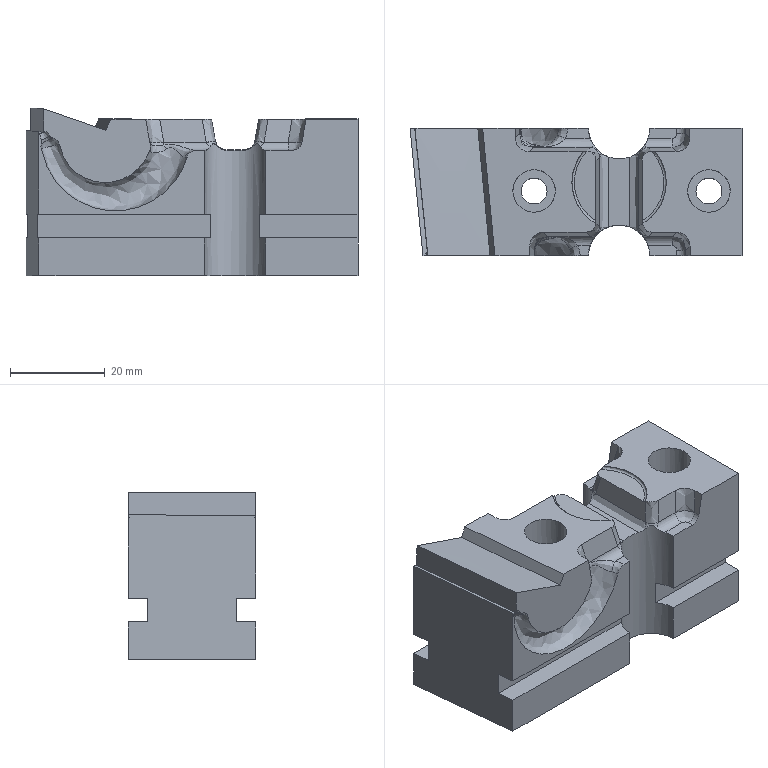Part | STEP file | P011002M006-000 | 1 solid | 108 faces | box 70.25 x 27 x 35.42 mm | volume 49386 mm3 | spline 51 | plane 39 | cylinder 12 | other 2 | cone 2 | torus 2 | commonest cylinder face diameters 4 x4 5.5 x2 9 x2 13 x2 20 x2